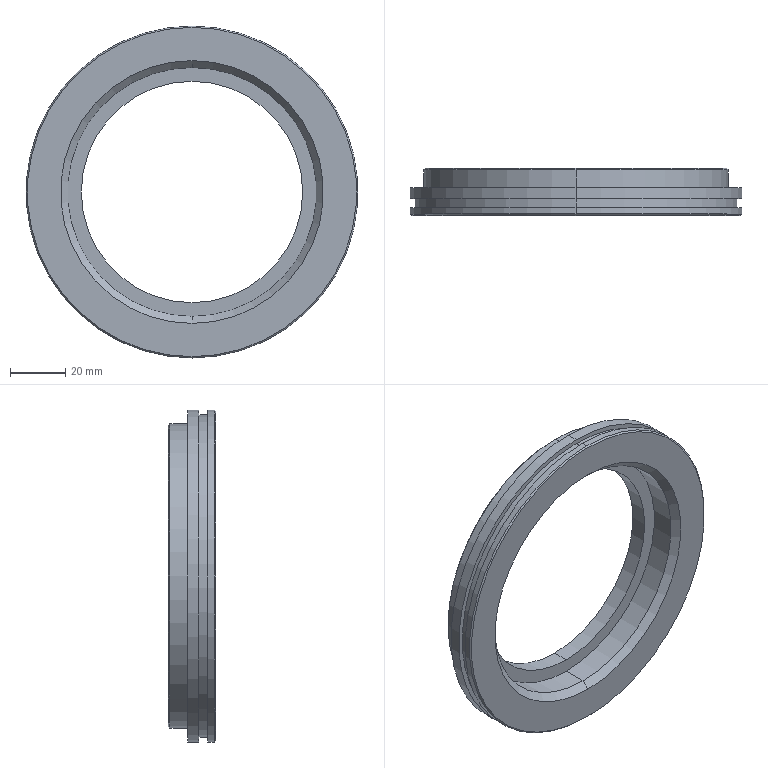Part | SolidWorks | features ICE 4, Chamfer 3, Extrusion 1, MoveFace 1 | 1 solid | 24 faces | box 120 x 17 x 120 mm | volume 76412 mm3 | cylinder 12 | cone 6 | plane 6 | commonest cylinder face diameters 120 x4 80 x2 90 x2 110 x2 116.5 x2
STEP:
#1=CARTESIAN_POINT('',(0.,2.5,45.));
#2=VERTEX_POINT('',#1);
#3=CARTESIAN_POINT('',(0.,2.5,-45.));
#4=VERTEX_POINT('',#3);
#5=CARTESIAN_POINT('',(0.,2.5,0.));
#6=DIRECTION('',(0.,-1.,0.));
#7=DIRECTION('',(0.,0.,1.));
#8=AXIS2_PLACEMENT_3D('',#5,#6,#7);
#9=CIRCLE('',#8,45.);
#10=EDGE_CURVE('',#2,#4,#9,.T.);
#11=ORIENTED_EDGE('',*,*,#10,.F.);
#12=CARTESIAN_POINT('',(0.,0.,47.5));
#13=VERTEX_POINT('',#12);
#14=CARTESIAN_POINT('',(0.,2.5,45.));
#15=DIRECTION('',(0.,-0.7071,0.7071));
#16=VECTOR('',#15,1000.);
#17=LINE('',#14,#16);
#18=EDGE_CURVE('',#2,#13,#17,.T.);
#19=ORIENTED_EDGE('',*,*,#18,.T.);
#20=CARTESIAN_POINT('',(0.,0.,-47.5));
#21=VERTEX_POINT('',#20);
#22=CARTESIAN_POINT('',(0.,0.,0.));
#23=DIRECTION('',(0.,1.,0.));
#24=DIRECTION('',(0.,0.,1.));
#25=AXIS2_PLACEMENT_3D('',#22,#23,#24);
#26=CIRCLE('',#25,47.5);
#27=EDGE_CURVE('',#21,#13,#26,.T.);
#28=ORIENTED_EDGE('',*,*,#27,.F.);
#29=CARTESIAN_POINT('',(0.,2.5,-45.));
#30=DIRECTION('',(0.,-0.7071,-0.7071));
#31=VECTOR('',#30,1000.);
#32=LINE('',#29,#31);
#33=EDGE_CURVE('',#4,#21,#32,.T.);
#34=ORIENTED_EDGE('',*,*,#33,.F.);
#35=EDGE_LOOP('',(#11,#19,#28,#34));
#36=FACE_OUTER_BOUND('',#35,.T.);
#37=CARTESIAN_POINT('',(0.,2.5,0.));
#38=DIRECTION('',(0.,-1.,0.));
#39=DIRECTION('',(0.,0.,-1.));
#40=AXIS2_PLACEMENT_3D('',#37,#38,#39);
#41=CONICAL_SURFACE('',#40,45.,0.7854);
#42=ADVANCED_FACE('',(#36),#41,.F.);
#43=CARTESIAN_POINT('',(0.,17.,54.5));
#44=VERTEX_POINT('',#43);
#45=CARTESIAN_POINT('',(0.,17.,-54.5));
#46=VERTEX_POINT('',#45);
#47=CARTESIAN_POINT('',(0.,17.,0.));
#48=DIRECTION('',(0.,1.,0.));
#49=DIRECTION('',(0.,0.,1.));
#50=AXIS2_PLACEMENT_3D('',#47,#48,#49);
#51=CIRCLE('',#50,54.5);
#52=EDGE_CURVE('',#44,#46,#51,.T.);
#53=ORIENTED_EDGE('',*,*,#52,.F.);
#54=CARTESIAN_POINT('',(0.,16.5,55.));
#55=VERTEX_POINT('',#54);
#56=CARTESIAN_POINT('',(0.,17.,54.5));
#57=DIRECTION('',(0.,-0.7071,0.7071));
#58=VECTOR('',#57,1000.);
#59=LINE('',#56,#58);
#60=EDGE_CURVE('',#44,#55,#59,.T.);
#61=ORIENTED_EDGE('',*,*,#60,.T.);
#62=CARTESIAN_POINT('',(0.,16.5,-55.));
#63=VERTEX_POINT('',#62);
#64=CARTESIAN_POINT('',(0.,16.5,0.));
#65=DIRECTION('',(0.,-1.,0.));
#66=DIRECTION('',(0.,0.,1.));
#67=AXIS2_PLACEMENT_3D('',#64,#65,#66);
#68=CIRCLE('',#67,55.);
#69=EDGE_CURVE('',#63,#55,#68,.T.);
#70=ORIENTED_EDGE('',*,*,#69,.F.);
#71=CARTESIAN_POINT('',(0.,17.,-54.5));
#72=DIRECTION('',(0.,-0.7071,-0.7071));
#73=VECTOR('',#72,1000.);
#74=LINE('',#71,#73);
#75=EDGE_CURVE('',#46,#63,#74,.T.);
#76=ORIENTED_EDGE('',*,*,#75,.F.);
#77=EDGE_LOOP('',(#53,#61,#70,#76));
#78=FACE_OUTER_BOUND('',#77,.T.);
#79=CARTESIAN_POINT('',(0.,17.,0.));
#80=DIRECTION('',(0.,-1.,0.));
#81=DIRECTION('',(0.,0.,-1.));
#82=AXIS2_PLACEMENT_3D('',#79,#80,#81);
#83=CONICAL_SURFACE('',#82,54.5,0.7854);
#84=ADVANCED_FACE('',(#78),#83,.T.);
#85=CARTESIAN_POINT('',(0.,0.,-59.5));
#86=VERTEX_POINT('',#85);
#87=CARTESIAN_POINT('',(0.,0.,59.5));
#88=VERTEX_POINT('',#87);
#89=CARTESIAN_POINT('',(0.,0.,0.));
#90=DIRECTION('',(0.,-1.,0.));
#91=DIRECTION('',(0.,0.,1.));
#92=AXIS2_PLACEMENT_3D('',#89,#90,#91);
#93=CIRCLE('',#92,59.5);
#94=EDGE_CURVE('',#86,#88,#93,.T.);
#95=ORIENTED_EDGE('',*,*,#94,.F.);
#96=CARTESIAN_POINT('',(0.,0.5,-60.));
#97=VERTEX_POINT('',#96);
#98=CARTESIAN_POINT('',(0.,0.5,-60.));
#99=DIRECTION('',(0.,0.7071,-0.7071));
#100=VECTOR('',#99,1000.);
#101=LINE('',#98,#100);
#102=EDGE_CURVE('',#86,#97,#101,.T.);
#103=ORIENTED_EDGE('',*,*,#102,.T.);
#104=CARTESIAN_POINT('',(0.,0.5,60.));
#105=VERTEX_POINT('',#104);
#106=CARTESIAN_POINT('',(0.,0.5,0.));
#107=DIRECTION('',(0.,1.,0.));
#108=DIRECTION('',(0.,0.,1.));
#109=AXIS2_PLACEMENT_3D('',#106,#107,#108);
#110=CIRCLE('',#109,60.);
#111=EDGE_CURVE('',#105,#97,#110,.T.);
#112=ORIENTED_EDGE('',*,*,#111,.F.);
#113=CARTESIAN_POINT('',(0.,0.5,60.));
#114=DIRECTION('',(0.,0.7071,0.7071));
#115=VECTOR('',#114,1000.);
#116=LINE('',#113,#115);
#117=EDGE_CURVE('',#88,#105,#116,.T.);
#118=ORIENTED_EDGE('',*,*,#117,.F.);
#119=EDGE_LOOP('',(#95,#103,#112,#118));
#120=FACE_OUTER_BOUND('',#119,.T.);
#121=CARTESIAN_POINT('',(0.,0.5,0.));
#122=DIRECTION('',(0.,1.,0.));
#123=DIRECTION('',(0.,0.,1.));
#124=AXIS2_PLACEMENT_3D('',#121,#122,#123);
#125=CONICAL_SURFACE('',#124,60.,0.7854);
#126=ADVANCED_FACE('',(#120),#125,.T.);
#127=CARTESIAN_POINT('',(0.,2.8,-58.25));
#128=VERTEX_POINT('',#127);
#129=CARTESIAN_POINT('',(0.,2.8,58.25));
#130=VERTEX_POINT('',#129);
#131=CARTESIAN_POINT('',(0.,2.8,0.));
#132=DIRECTION('',(0.,-1.,0.));
#133=DIRECTION('',(0.,0.,-1.));
#134=AXIS2_PLACEMENT_3D('',#131,#132,#133);
#135=CIRCLE('',#134,58.25);
#136=EDGE_CURVE('',#128,#130,#135,.T.);
#137=ORIENTED_EDGE('',*,*,#136,.F.);
#138=CARTESIAN_POINT('',(0.,6.,-58.25));
#139=VERTEX_POINT('',#138);
#140=CARTESIAN_POINT('',(0.,2.8,-58.25));
#141=DIRECTION('',(0.,1.,0.));
#142=VECTOR('',#141,1000.);
#143=LINE('',#140,#142);
#144=EDGE_CURVE('',#128,#139,#143,.T.);
#145=ORIENTED_EDGE('',*,*,#144,.T.);
#146=CARTESIAN_POINT('',(0.,6.,58.25));
#147=VERTEX_POINT('',#146);
#148=CARTESIAN_POINT('',(0.,6.,0.));
#149=DIRECTION('',(0.,-1.,0.));
#150=DIRECTION('',(0.,0.,-1.));
#151=AXIS2_PLACEMENT_3D('',#148,#149,#150);
#152=CIRCLE('',#151,58.25);
#153=EDGE_CURVE('',#139,#147,#152,.T.);
#154=ORIENTED_EDGE('',*,*,#153,.T.);
#155=CARTESIAN_POINT('',(0.,2.8,58.25));
#156=DIRECTION('',(0.,1.,0.));
#157=VECTOR('',#156,1000.);
#158=LINE('',#155,#157);
#159=EDGE_CURVE('',#130,#147,#158,.T.);
#160=ORIENTED_EDGE('',*,*,#159,.F.);
#161=EDGE_LOOP('',(#137,#145,#154,#160));
#162=FACE_OUTER_BOUND('',#161,.T.);
#163=CARTESIAN_POINT('',(0.,2.8,0.));
#164=DIRECTION('',(0.,1.,0.));
#165=DIRECTION('',(0.,0.,1.));
#166=AXIS2_PLACEMENT_3D('',#163,#164,#165);
#167=CYLINDRICAL_SURFACE('',#166,58.25);
#168=ADVANCED_FACE('',(#162),#167,.T.);
#169=CARTESIAN_POINT('',(0.,11.,45.));
#170=VERTEX_POINT('',#169);
#171=CARTESIAN_POINT('',(0.,11.,-45.));
#172=VERTEX_POINT('',#171);
#173=CARTESIAN_POINT('',(0.,11.,0.));
#174=DIRECTION('',(0.,-1.,0.));
#175=DIRECTION('',(0.,0.,-1.));
#176=AXIS2_PLACEMENT_3D('',#173,#174,#175);
#177=CIRCLE('',#176,45.);
#178=EDGE_CURVE('',#170,#172,#177,.T.);
#179=ORIENTED_EDGE('',*,*,#178,.F.);
#180=CARTESIAN_POINT('',(0.,11.,45.));
#181=DIRECTION('',(0.,-1.,0.));
#182=VECTOR('',#181,1000.);
#183=LINE('',#180,#182);
#184=EDGE_CURVE('',#170,#2,#183,.T.);
#185=ORIENTED_EDGE('',*,*,#184,.T.);
#186=ORIENTED_EDGE('',*,*,#10,.T.);
#187=CARTESIAN_POINT('',(0.,11.,-45.));
#188=DIRECTION('',(0.,-1.,0.));
#189=VECTOR('',#188,1000.);
#190=LINE('',#187,#189);
#191=EDGE_CURVE('',#172,#4,#190,.T.);
#192=ORIENTED_EDGE('',*,*,#191,.F.);
#193=EDGE_LOOP('',(#179,#185,#186,#192));
#194=FACE_OUTER_BOUND('',#193,.T.);
#195=CARTESIAN_POINT('',(0.,11.,0.));
#196=DIRECTION('',(0.,-1.,0.));
#197=DIRECTION('',(0.,0.,-1.));
#198=AXIS2_PLACEMENT_3D('',#195,#196,#197);
#199=CYLINDRICAL_SURFACE('',#198,45.);
#200=ADVANCED_FACE('',(#194),#199,.F.);
#201=ORIENTED_EDGE('',*,*,#69,.T.);
#202=CARTESIAN_POINT('',(0.,10.,55.));
#203=VERTEX_POINT('',#202);
#204=CARTESIAN_POINT('',(0.,17.,55.));
#205=DIRECTION('',(0.,-1.,0.));
#206=VECTOR('',#205,1000.);
#207=LINE('',#204,#206);
#208=EDGE_CURVE('',#55,#203,#207,.T.);
#209=ORIENTED_EDGE('',*,*,#208,.T.);
#210=CARTESIAN_POINT('',(0.,10.,-55.));
#211=VERTEX_POINT('',#210);
#212=CARTESIAN_POINT('',(0.,10.,0.));
#213=DIRECTION('',(0.,1.,0.));
#214=DIRECTION('',(0.,0.,1.));
#215=AXIS2_PLACEMENT_3D('',#212,#213,#214);
#216=CIRCLE('',#215,55.);
#217=EDGE_CURVE('',#203,#211,#216,.T.);
#218=ORIENTED_EDGE('',*,*,#217,.T.);
#219=CARTESIAN_POINT('',(0.,17.,-55.));
#220=DIRECTION('',(0.,-1.,0.));
#221=VECTOR('',#220,1000.);
#222=LINE('',#219,#221);
#223=EDGE_CURVE('',#63,#211,#222,.T.);
#224=ORIENTED_EDGE('',*,*,#223,.F.);
#225=EDGE_LOOP('',(#201,#209,#218,#224));
#226=FACE_OUTER_BOUND('',#225,.T.);
#227=CARTESIAN_POINT('',(0.,17.,0.));
#228=DIRECTION('',(0.,-1.,0.));
#229=DIRECTION('',(0.,0.,-1.));
#230=AXIS2_PLACEMENT_3D('',#227,#228,#229);
#231=CYLINDRICAL_SURFACE('',#230,55.);
#232=ADVANCED_FACE('',(#226),#231,.T.);
#233=CARTESIAN_POINT('',(0.,2.8,-60.));
#234=VERTEX_POINT('',#233);
#235=CARTESIAN_POINT('',(0.,2.8,60.));
#236=VERTEX_POINT('',#235);
#237=CARTESIAN_POINT('',(0.,2.8,0.));
#238=DIRECTION('',(0.,-1.,0.));
#239=DIRECTION('',(0.,0.,-1.));
#240=AXIS2_PLACEMENT_3D('',#237,#238,#239);
#241=CIRCLE('',#240,60.);
#242=EDGE_CURVE('',#234,#236,#241,.T.);
#243=ORIENTED_EDGE('',*,*,#242,.T.);
#244=CARTESIAN_POINT('',(0.,10.,60.));
#245=DIRECTION('',(0.,-1.,0.));
#246=VECTOR('',#245,1000.);
#247=LINE('',#244,#246);
#248=EDGE_CURVE('',#236,#105,#247,.T.);
#249=ORIENTED_EDGE('',*,*,#248,.T.);
#250=ORIENTED_EDGE('',*,*,#111,.T.);
#251=CARTESIAN_POINT('',(0.,10.,-60.));
#252=DIRECTION('',(0.,-1.,0.));
#253=VECTOR('',#252,1000.);
#254=LINE('',#251,#253);
#255=EDGE_CURVE('',#234,#97,#254,.T.);
#256=ORIENTED_EDGE('',*,*,#255,.F.);
#257=EDGE_LOOP('',(#243,#249,#250,#256));
#258=FACE_OUTER_BOUND('',#257,.T.);
#259=CARTESIAN_POINT('',(0.,10.,0.));
#260=DIRECTION('',(0.,-1.,0.));
#261=DIRECTION('',(0.,0.,-1.));
#262=AXIS2_PLACEMENT_3D('',#259,#260,#261);
#263=CYLINDRICAL_SURFACE('',#262,60.);
#264=ADVANCED_FACE('',(#258),#263,.T.);
#265=CARTESIAN_POINT('',(0.,11.,-40.));
#266=VERTEX_POINT('',#265);
#267=CARTESIAN_POINT('',(0.,11.,40.));
#268=VERTEX_POINT('',#267);
#269=CARTESIAN_POINT('',(0.,11.,0.));
#270=DIRECTION('',(0.,1.,0.));
#271=DIRECTION('',(0.,0.,-1.));
#272=AXIS2_PLACEMENT_3D('',#269,#270,#271);
#273=CIRCLE('',#272,40.);
#274=EDGE_CURVE('',#266,#268,#273,.T.);
#275=ORIENTED_EDGE('',*,*,#274,.F.);
#276=CARTESIAN_POINT('',(0.,17.,-40.));
#277=VERTEX_POINT('',#276);
#278=CARTESIAN_POINT('',(0.,0.,-40.));
#279=DIRECTION('',(0.,1.,0.));
#280=VECTOR('',#279,1000.);
#281=LINE('',#278,#280);
#282=EDGE_CURVE('',#266,#277,#281,.T.);
#283=ORIENTED_EDGE('',*,*,#282,.T.);
#284=CARTESIAN_POINT('',(0.,17.,40.));
#285=VERTEX_POINT('',#284);
#286=CARTESIAN_POINT('',(0.,17.,0.));
#287=DIRECTION('',(0.,1.,0.));
#288=DIRECTION('',(0.,0.,1.));
#289=AXIS2_PLACEMENT_3D('',#286,#287,#288);
#290=CIRCLE('',#289,40.);
#291=EDGE_CURVE('',#277,#285,#290,.T.);
#292=ORIENTED_EDGE('',*,*,#291,.T.);
#293=CARTESIAN_POINT('',(0.,0.,40.));
#294=DIRECTION('',(0.,1.,0.));
#295=VECTOR('',#294,1000.);
#296=LINE('',#293,#295);
#297=EDGE_CURVE('',#268,#285,#296,.T.);
#298=ORIENTED_EDGE('',*,*,#297,.F.);
#299=EDGE_LOOP('',(#275,#283,#292,#298));
#300=FACE_OUTER_BOUND('',#299,.T.);
#301=CARTESIAN_POINT('',(0.,0.,0.));
#302=DIRECTION('',(0.,1.,0.));
#303=DIRECTION('',(0.,0.,1.));
#304=AXIS2_PLACEMENT_3D('',#301,#302,#303);
#305=CYLINDRICAL_SURFACE('',#304,40.);
#306=ADVANCED_FACE('',(#300),#305,.F.);
#307=CARTESIAN_POINT('',(0.,10.,60.));
#308=VERTEX_POINT('',#307);
#309=CARTESIAN_POINT('',(0.,10.,-60.));
#310=VERTEX_POINT('',#309);
#311=CARTESIAN_POINT('',(0.,10.,0.));
#312=DIRECTION('',(0.,1.,0.));
#313=DIRECTION('',(0.,0.,1.));
#314=AXIS2_PLACEMENT_3D('',#311,#312,#313);
#315=CIRCLE('',#314,60.);
#316=EDGE_CURVE('',#308,#310,#315,.T.);
#317=ORIENTED_EDGE('',*,*,#316,.F.);
#318=CARTESIAN_POINT('',(0.,6.,60.));
#319=VERTEX_POINT('',#318);
#320=CARTESIAN_POINT('',(0.,9.,60.));
#321=DIRECTION('',(0.,-1.,0.));
#322=VECTOR('',#321,1000.);
#323=LINE('',#320,#322);
#324=EDGE_CURVE('',#308,#319,#323,.T.);
#325=ORIENTED_EDGE('',*,*,#324,.T.);
#326=CARTESIAN_POINT('',(0.,6.,-60.));
#327=VERTEX_POINT('',#326);
#328=CARTESIAN_POINT('',(0.,6.,0.));
#329=DIRECTION('',(0.,-1.,0.));
#330=DIRECTION('',(0.,0.,-1.));
#331=AXIS2_PLACEMENT_3D('',#328,#329,#330);
#332=CIRCLE('',#331,60.);
#333=EDGE_CURVE('',#327,#319,#332,.T.);
#334=ORIENTED_EDGE('',*,*,#333,.F.);
#335=CARTESIAN_POINT('',(0.,9.,-60.));
#336=DIRECTION('',(0.,-1.,0.));
#337=VECTOR('',#336,1000.);
#338=LINE('',#335,#337);
#339=EDGE_CURVE('',#310,#327,#338,.T.);
#340=ORIENTED_EDGE('',*,*,#339,.F.);
#341=EDGE_LOOP('',(#317,#325,#334,#340));
#342=FACE_OUTER_BOUND('',#341,.T.);
#343=CARTESIAN_POINT('',(0.,9.,0.));
#344=DIRECTION('',(0.,-1.,0.));
#345=DIRECTION('',(0.,0.,-1.));
#346=AXIS2_PLACEMENT_3D('',#343,#344,#345);
#347=CYLINDRICAL_SURFACE('',#346,60.);
#348=ADVANCED_FACE('',(#342),#347,.T.);
#349=ORIENTED_EDGE('',*,*,#324,.F.);
#350=CARTESIAN_POINT('',(0.,10.,0.));
#351=DIRECTION('',(0.,1.,0.));
#352=DIRECTION('',(0.,0.,1.));
#353=AXIS2_PLACEMENT_3D('',#350,#351,#352);
#354=CIRCLE('',#353,60.);
#355=EDGE_CURVE('',#310,#308,#354,.T.);
#356=ORIENTED_EDGE('',*,*,#355,.F.);
#357=ORIENTED_EDGE('',*,*,#339,.T.);
#358=CARTESIAN_POINT('',(0.,6.,0.));
#359=DIRECTION('',(0.,-1.,0.));
#360=DIRECTION('',(0.,0.,-1.));
#361=AXIS2_PLACEMENT_3D('',#358,#359,#360);
#362=CIRCLE('',#361,60.);
#363=EDGE_CURVE('',#319,#327,#362,.T.);
#364=ORIENTED_EDGE('',*,*,#363,.F.);
#365=EDGE_LOOP('',(#349,#356,#357,#364));
#366=FACE_OUTER_BOUND('',#365,.T.);
#367=CARTESIAN_POINT('',(0.,9.,0.));
#368=DIRECTION('',(0.,-1.,0.));
#369=DIRECTION('',(0.,0.,-1.));
#370=AXIS2_PLACEMENT_3D('',#367,#368,#369);
#371=CYLINDRICAL_SURFACE('',#370,60.);
#372=ADVANCED_FACE('',(#366),#371,.T.);
#373=ORIENTED_EDGE('',*,*,#282,.F.);
#374=CARTESIAN_POINT('',(0.,11.,0.));
#375=DIRECTION('',(0.,1.,0.));
#376=DIRECTION('',(0.,0.,-1.));
#377=AXIS2_PLACEMENT_3D('',#374,#375,#376);
#378=CIRCLE('',#377,40.);
#379=EDGE_CURVE('',#268,#266,#378,.T.);
#380=ORIENTED_EDGE('',*,*,#379,.F.);
#381=ORIENTED_EDGE('',*,*,#297,.T.);
#382=CARTESIAN_POINT('',(0.,17.,0.));
#383=DIRECTION('',(0.,1.,0.));
#384=DIRECTION('',(0.,0.,1.));
#385=AXIS2_PLACEMENT_3D('',#382,#383,#384);
#386=CIRCLE('',#385,40.);
#387=EDGE_CURVE('',#285,#277,#386,.T.);
#388=ORIENTED_EDGE('',*,*,#387,.T.);
#389=EDGE_LOOP('',(#373,#380,#381,#388));
#390=FACE_OUTER_BOUND('',#389,.T.);
#391=CARTESIAN_POINT('',(0.,0.,0.));
#392=DIRECTION('',(0.,1.,0.));
#393=DIRECTION('',(0.,0.,1.));
#394=AXIS2_PLACEMENT_3D('',#391,#392,#393);
#395=CYLINDRICAL_SURFACE('',#394,40.);
#396=ADVANCED_FACE('',(#390),#395,.F.);
#397=ORIENTED_EDGE('',*,*,#248,.F.);
#398=CARTESIAN_POINT('',(0.,2.8,0.));
#399=DIRECTION('',(0.,-1.,0.));
#400=DIRECTION('',(0.,0.,-1.));
#401=AXIS2_PLACEMENT_3D('',#398,#399,#400);
#402=CIRCLE('',#401,60.);
#403=EDGE_CURVE('',#236,#234,#402,.T.);
#404=ORIENTED_EDGE('',*,*,#403,.T.);
#405=ORIENTED_EDGE('',*,*,#255,.T.);
#406=CARTESIAN_POINT('',(0.,0.5,0.));
#407=DIRECTION('',(0.,1.,0.));
#408=DIRECTION('',(0.,0.,1.));
#409=AXIS2_PLACEMENT_3D('',#406,#407,#408);
#410=CIRCLE('',#409,60.);
#411=EDGE_CURVE('',#97,#105,#410,.T.);
#412=ORIENTED_EDGE('',*,*,#411,.T.);
#413=EDGE_LOOP('',(#397,#404,#405,#412));
#414=FACE_OUTER_BOUND('',#413,.T.);
#415=CARTESIAN_POINT('',(0.,10.,0.));
#416=DIRECTION('',(0.,-1.,0.));
#417=DIRECTION('',(0.,0.,-1.));
#418=AXIS2_PLACEMENT_3D('',#415,#416,#417);
#419=CYLINDRICAL_SURFACE('',#418,60.);
#420=ADVANCED_FACE('',(#414),#419,.T.);
#421=CARTESIAN_POINT('',(0.,10.,0.));
#422=DIRECTION('',(0.,1.,0.));
#423=DIRECTION('',(0.,0.,1.));
#424=AXIS2_PLACEMENT_3D('',#421,#422,#423);
#425=CIRCLE('',#424,55.);
#426=EDGE_CURVE('',#211,#203,#425,.T.);
#427=ORIENTED_EDGE('',*,*,#426,.F.);
#428=ORIENTED_EDGE('',*,*,#217,.F.);
#429=EDGE_LOOP('',(#427,#428));
#430=FACE_BOUND('',#429,.T.);
#431=ORIENTED_EDGE('',*,*,#355,.T.);
#432=ORIENTED_EDGE('',*,*,#316,.T.);
#433=EDGE_LOOP('',(#431,#432));
#434=FACE_OUTER_BOUND('',#433,.T.);
#435=CARTESIAN_POINT('',(0.,10.,0.));
#436=DIRECTION('',(0.,1.,0.));
#437=DIRECTION('',(0.,0.,1.));
#438=AXIS2_PLACEMENT_3D('',#435,#436,#437);
#439=PLANE('',#438);
#440=ADVANCED_FACE('',(#430,#434),#439,.T.);
#441=ORIENTED_EDGE('',*,*,#27,.T.);
#442=CARTESIAN_POINT('',(0.,0.,0.));
#443=DIRECTION('',(0.,1.,0.));
#444=DIRECTION('',(0.,0.,1.));
#445=AXIS2_PLACEMENT_3D('',#442,#443,#444);
#446=CIRCLE('',#445,47.5);
#447=EDGE_CURVE('',#13,#21,#446,.T.);
#448=ORIENTED_EDGE('',*,*,#447,.T.);
#449=EDGE_LOOP('',(#441,#448));
#450=FACE_BOUND('',#449,.T.);
#451=CARTESIAN_POINT('',(0.,0.,0.));
#452=DIRECTION('',(0.,-1.,0.));
#453=DIRECTION('',(0.,0.,1.));
#454=AXIS2_PLACEMENT_3D('',#451,#452,#453);
#455=CIRCLE('',#454,59.5);
#456=EDGE_CURVE('',#88,#86,#455,.T.);
#457=ORIENTED_EDGE('',*,*,#456,.T.);
#458=ORIENTED_EDGE('',*,*,#94,.T.);
#459=EDGE_LOOP('',(#457,#458));
#460=FACE_OUTER_BOUND('',#459,.T.);
#461=CARTESIAN_POINT('',(0.,0.,0.));
#462=DIRECTION('',(0.,1.,0.));
#463=DIRECTION('',(0.,0.,1.));
#464=AXIS2_PLACEMENT_3D('',#461,#462,#463);
#465=PLANE('',#464);
#466=ADVANCED_FACE('',(#450,#460),#465,.F.);
#467=ORIENTED_EDGE('',*,*,#208,.F.);
#468=CARTESIAN_POINT('',(0.,16.5,0.));
#469=DIRECTION('',(0.,-1.,0.));
#470=DIRECTION('',(0.,0.,1.));
#471=AXIS2_PLACEMENT_3D('',#468,#469,#470);
#472=CIRCLE('',#471,55.);
#473=EDGE_CURVE('',#55,#63,#472,.T.);
#474=ORIENTED_EDGE('',*,*,#473,.T.);
#475=ORIENTED_EDGE('',*,*,#223,.T.);
#476=ORIENTED_EDGE('',*,*,#426,.T.);
#477=EDGE_LOOP('',(#467,#474,#475,#476));
#478=FACE_OUTER_BOUND('',#477,.T.);
#479=CARTESIAN_POINT('',(0.,17.,0.));
#480=DIRECTION('',(0.,-1.,0.));
#481=DIRECTION('',(0.,0.,-1.));
#482=AXIS2_PLACEMENT_3D('',#479,#480,#481);
#483=CYLINDRICAL_SURFACE('',#482,55.);
#484=ADVANCED_FACE('',(#478),#483,.T.);
#485=CARTESIAN_POINT('',(0.,17.,0.));
#486=DIRECTION('',(0.,1.,0.));
#487=DIRECTION('',(0.,0.,1.));
#488=AXIS2_PLACEMENT_3D('',#485,#486,#487);
#489=CIRCLE('',#488,54.5);
#490=EDGE_CURVE('',#46,#44,#489,.T.);
#491=ORIENTED_EDGE('',*,*,#490,.T.);
#492=ORIENTED_EDGE('',*,*,#52,.T.);
#493=EDGE_LOOP('',(#491,#492));
#494=FACE_OUTER_BOUND('',#493,.T.);
#495=ORIENTED_EDGE('',*,*,#387,.F.);
#496=ORIENTED_EDGE('',*,*,#291,.F.);
#497=EDGE_LOOP('',(#495,#496));
#498=FACE_BOUND('',#497,.T.);
#499=CARTESIAN_POINT('',(0.,17.,0.));
#500=DIRECTION('',(0.,1.,0.));
#501=DIRECTION('',(0.,0.,1.));
#502=AXIS2_PLACEMENT_3D('',#499,#500,#501);
#503=PLANE('',#502);
#504=ADVANCED_FACE('',(#494,#498),#503,.T.);
#505=CARTESIAN_POINT('',(0.,11.,0.));
#506=DIRECTION('',(0.,-1.,0.));
#507=DIRECTION('',(0.,0.,-1.));
#508=AXIS2_PLACEMENT_3D('',#505,#506,#507);
#509=CIRCLE('',#508,45.);
#510=EDGE_CURVE('',#172,#170,#509,.T.);
#511=ORIENTED_EDGE('',*,*,#510,.T.);
#512=ORIENTED_EDGE('',*,*,#178,.T.);
#513=EDGE_LOOP('',(#511,#512));
#514=FACE_OUTER_BOUND('',#513,.T.);
#515=ORIENTED_EDGE('',*,*,#379,.T.);
#516=ORIENTED_EDGE('',*,*,#274,.T.);
#517=EDGE_LOOP('',(#515,#516));
#518=FACE_BOUND('',#517,.T.);
#519=CARTESIAN_POINT('',(0.,11.,0.));
#520=DIRECTION('',(0.,-1.,0.));
#521=DIRECTION('',(0.,0.,-1.));
#522=AXIS2_PLACEMENT_3D('',#519,#520,#521);
#523=PLANE('',#522);
#524=ADVANCED_FACE('',(#514,#518),#523,.T.);
#525=ORIENTED_EDGE('',*,*,#184,.F.);
#526=ORIENTED_EDGE('',*,*,#510,.F.);
#527=ORIENTED_EDGE('',*,*,#191,.T.);
#528=CARTESIAN_POINT('',(0.,2.5,0.));
#529=DIRECTION('',(0.,-1.,0.));
#530=DIRECTION('',(0.,0.,1.));
#531=AXIS2_PLACEMENT_3D('',#528,#529,#530);
#532=CIRCLE('',#531,45.);
#533=EDGE_CURVE('',#4,#2,#532,.T.);
#534=ORIENTED_EDGE('',*,*,#533,.T.);
#535=EDGE_LOOP('',(#525,#526,#527,#534));
#536=FACE_OUTER_BOUND('',#535,.T.);
#537=CARTESIAN_POINT('',(0.,11.,0.));
#538=DIRECTION('',(0.,-1.,0.));
#539=DIRECTION('',(0.,0.,-1.));
#540=AXIS2_PLACEMENT_3D('',#537,#538,#539);
#541=CYLINDRICAL_SURFACE('',#540,45.);
#542=ADVANCED_FACE('',(#536),#541,.F.);
#543=CARTESIAN_POINT('',(0.,2.8,0.));
#544=DIRECTION('',(0.,-1.,0.));
#545=DIRECTION('',(0.,0.,-1.));
#546=AXIS2_PLACEMENT_3D('',#543,#544,#545);
#547=CIRCLE('',#546,58.25);
#548=EDGE_CURVE('',#130,#128,#547,.T.);
#549=ORIENTED_EDGE('',*,*,#548,.T.);
#550=ORIENTED_EDGE('',*,*,#136,.T.);
#551=EDGE_LOOP('',(#549,#550));
#552=FACE_BOUND('',#551,.T.);
#553=ORIENTED_EDGE('',*,*,#242,.F.);
#554=ORIENTED_EDGE('',*,*,#403,.F.);
#555=EDGE_LOOP('',(#553,#554));
#556=FACE_OUTER_BOUND('',#555,.T.);
#557=CARTESIAN_POINT('',(0.,2.8,0.));
#558=DIRECTION('',(0.,-1.,0.));
#559=DIRECTION('',(0.,0.,-1.));
#560=AXIS2_PLACEMENT_3D('',#557,#558,#559);
#561=PLANE('',#560);
#562=ADVANCED_FACE('',(#552,#556),#561,.F.);
#563=CARTESIAN_POINT('',(0.,6.,0.));
#564=DIRECTION('',(0.,-1.,0.));
#565=DIRECTION('',(0.,0.,-1.));
#566=AXIS2_PLACEMENT_3D('',#563,#564,#565);
#567=CIRCLE('',#566,58.25);
#568=EDGE_CURVE('',#147,#139,#567,.T.);
#569=ORIENTED_EDGE('',*,*,#568,.F.);
#570=ORIENTED_EDGE('',*,*,#153,.F.);
#571=EDGE_LOOP('',(#569,#570));
#572=FACE_BOUND('',#571,.T.);
#573=ORIENTED_EDGE('',*,*,#333,.T.);
#574=ORIENTED_EDGE('',*,*,#363,.T.);
#575=EDGE_LOOP('',(#573,#574));
#576=FACE_OUTER_BOUND('',#575,.T.);
#577=CARTESIAN_POINT('',(0.,6.,0.));
#578=DIRECTION('',(0.,-1.,0.));
#579=DIRECTION('',(0.,0.,-1.));
#580=AXIS2_PLACEMENT_3D('',#577,#578,#579);
#581=PLANE('',#580);
#582=ADVANCED_FACE('',(#572,#576),#581,.T.);
#583=ORIENTED_EDGE('',*,*,#144,.F.);
#584=ORIENTED_EDGE('',*,*,#548,.F.);
#585=ORIENTED_EDGE('',*,*,#159,.T.);
#586=ORIENTED_EDGE('',*,*,#568,.T.);
#587=EDGE_LOOP('',(#583,#584,#585,#586));
#588=FACE_OUTER_BOUND('',#587,.T.);
#589=CARTESIAN_POINT('',(0.,2.8,0.));
#590=DIRECTION('',(0.,1.,0.));
#591=DIRECTION('',(0.,0.,1.));
#592=AXIS2_PLACEMENT_3D('',#589,#590,#591);
#593=CYLINDRICAL_SURFACE('',#592,58.25);
#594=ADVANCED_FACE('',(#588),#593,.T.);
#595=ORIENTED_EDGE('',*,*,#102,.F.);
#596=ORIENTED_EDGE('',*,*,#456,.F.);
#597=ORIENTED_EDGE('',*,*,#117,.T.);
#598=ORIENTED_EDGE('',*,*,#411,.F.);
#599=EDGE_LOOP('',(#595,#596,#597,#598));
#600=FACE_OUTER_BOUND('',#599,.T.);
#601=CARTESIAN_POINT('',(0.,0.5,0.));
#602=DIRECTION('',(0.,1.,0.));
#603=DIRECTION('',(0.,0.,1.));
#604=AXIS2_PLACEMENT_3D('',#601,#602,#603);
#605=CONICAL_SURFACE('',#604,60.,0.7854);
#606=ADVANCED_FACE('',(#600),#605,.T.);
#607=ORIENTED_EDGE('',*,*,#60,.F.);
#608=ORIENTED_EDGE('',*,*,#490,.F.);
#609=ORIENTED_EDGE('',*,*,#75,.T.);
#610=ORIENTED_EDGE('',*,*,#473,.F.);
#611=EDGE_LOOP('',(#607,#608,#609,#610));
#612=FACE_OUTER_BOUND('',#611,.T.);
#613=CARTESIAN_POINT('',(0.,17.,0.));
#614=DIRECTION('',(0.,-1.,0.));
#615=DIRECTION('',(0.,0.,-1.));
#616=AXIS2_PLACEMENT_3D('',#613,#614,#615);
#617=CONICAL_SURFACE('',#616,54.5,0.7854);
#618=ADVANCED_FACE('',(#612),#617,.T.);
#619=ORIENTED_EDGE('',*,*,#18,.F.);
#620=ORIENTED_EDGE('',*,*,#533,.F.);
#621=ORIENTED_EDGE('',*,*,#33,.T.);
#622=ORIENTED_EDGE('',*,*,#447,.F.);
#623=EDGE_LOOP('',(#619,#620,#621,#622));
#624=FACE_OUTER_BOUND('',#623,.T.);
#625=CARTESIAN_POINT('',(0.,2.5,0.));
#626=DIRECTION('',(0.,-1.,0.));
#627=DIRECTION('',(0.,0.,-1.));
#628=AXIS2_PLACEMENT_3D('',#625,#626,#627);
#629=CONICAL_SURFACE('',#628,45.,0.7854);
#630=ADVANCED_FACE('',(#624),#629,.F.);
#631=CLOSED_SHELL('',(#42,#84,#126,#168,#200,#232,#264,#306,#348,#372,#396,#420,#440,#466,#484,#504,#524,#542,#562,#582,#594,#606,#618,#630));
#632=MANIFOLD_SOLID_BREP('',#631);
#633=CARTESIAN_POINT('',(0.,0.,0.));
#634=DIRECTION('',(0.,0.,1.));
#635=DIRECTION('',(1.,0.,0.));
#636=AXIS2_PLACEMENT_3D('',#633,#634,#635);
#637=(LENGTH_UNIT()NAMED_UNIT(*)SI_UNIT(.MILLI.,.METRE.));
#638=UNCERTAINTY_MEASURE_WITH_UNIT(LENGTH_MEASURE(0.00001),#637,'','');
#639=(NAMED_UNIT(*)PLANE_ANGLE_UNIT()SI_UNIT($,.RADIAN.));
#640=(NAMED_UNIT(*)SI_UNIT($,.STERADIAN.)SOLID_ANGLE_UNIT());
#641=(GEOMETRIC_REPRESENTATION_CONTEXT(3)GLOBAL_UNCERTAINTY_ASSIGNED_CONTEXT((#638))GLOBAL_UNIT_ASSIGNED_CONTEXT((#637,#639,#640))REPRESENTATION_CONTEXT('',''));
#642=ADVANCED_BREP_SHAPE_REPRESENTATION('',(#632,#636),#641);